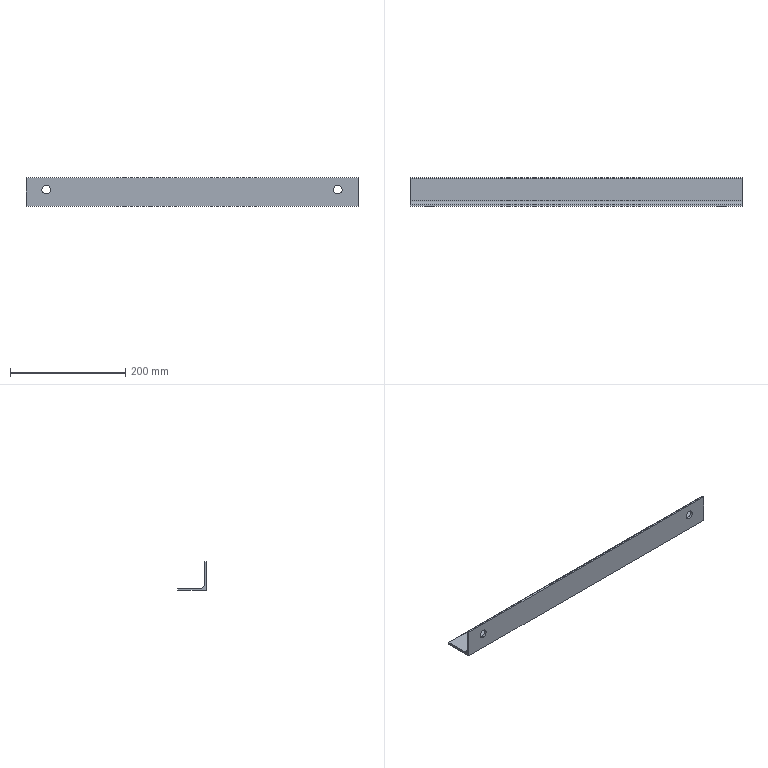Part | STEP file | 电柜通道角钢1_Default<As Machined> | 1 solid | 15 faces | box 575 x 50 x 50 mm | volume 222682 mm3 | plane 8 | cylinder 7 | commonest cylinder face diameters 15 x4 2.66 x2 11 x1
STEP:
#1=CARTESIAN_POINT('',(0.,0.,0.));
#2=DIRECTION('',(0.,0.,1.));
#3=DIRECTION('',(1.,0.,0.));
#4=AXIS2_PLACEMENT_3D('',#1,#2,#3);
#5=CARTESIAN_POINT('',(-252.5,0.,36.585));
#6=VERTEX_POINT('',#5);
#7=CARTESIAN_POINT('',(-252.5,4.,36.585));
#8=VERTEX_POINT('',#7);
#9=CARTESIAN_POINT('',(-252.5,-6.,36.585));
#10=DIRECTION('',(0.,1.,0.));
#11=VECTOR('',#10,1.);
#12=LINE('',#9,#11);
#13=CARTESIAN_POINT('',(-252.5,-6.,29.085));
#14=DIRECTION('',(0.,1.,0.));
#15=DIRECTION('',(0.,0.,1.));
#16=AXIS2_PLACEMENT_3D('',#13,#14,#15);
#17=CYLINDRICAL_SURFACE('',#16,7.5);
#18=CARTESIAN_POINT('',(6.283,0.));
#19=DIRECTION('',(0.,1.));
#20=VECTOR('',#19,1.);
#21=LINE('',#18,#20);
#22=(GEOMETRIC_REPRESENTATION_CONTEXT(2)PARAMETRIC_REPRESENTATION_CONTEXT()REPRESENTATION_CONTEXT('',''));
#23=DEFINITIONAL_REPRESENTATION('',(#21),#22);
#24=PCURVE('',#17,#23);
#25=CARTESIAN_POINT('',(-252.5,-6.,29.085));
#26=DIRECTION('',(0.,1.,0.));
#27=DIRECTION('',(0.,0.,1.));
#28=AXIS2_PLACEMENT_3D('',#25,#26,#27);
#29=CYLINDRICAL_SURFACE('',#28,7.5);
#30=CARTESIAN_POINT('',(0.,0.));
#31=DIRECTION('',(0.,1.));
#32=VECTOR('',#31,1.);
#33=LINE('',#30,#32);
#34=(GEOMETRIC_REPRESENTATION_CONTEXT(2)PARAMETRIC_REPRESENTATION_CONTEXT()REPRESENTATION_CONTEXT('',''));
#35=DEFINITIONAL_REPRESENTATION('',(#33),#34);
#36=PCURVE('',#29,#35);
#37=SURFACE_CURVE('',#12,(#24,#36),.PCURVE_S1.);
#38=EDGE_CURVE('',#6,#8,#37,.T.);
#39=ORIENTED_EDGE('',*,*,#38,.T.);
#40=CARTESIAN_POINT('',(-252.5,4.,21.585));
#41=VERTEX_POINT('',#40);
#42=CARTESIAN_POINT('',(-252.5,4.,29.085));
#43=DIRECTION('',(0.,1.,0.));
#44=DIRECTION('',(0.,0.,1.));
#45=AXIS2_PLACEMENT_3D('',#42,#43,#44);
#46=CIRCLE('',#45,7.5);
#47=CARTESIAN_POINT('',(0.,10.));
#48=DIRECTION('',(1.,0.));
#49=VECTOR('',#48,1.);
#50=LINE('',#47,#49);
#51=(GEOMETRIC_REPRESENTATION_CONTEXT(2)PARAMETRIC_REPRESENTATION_CONTEXT()REPRESENTATION_CONTEXT('',''));
#52=DEFINITIONAL_REPRESENTATION('',(#50),#51);
#53=PCURVE('',#17,#52);
#54=CARTESIAN_POINT('',(287.5,4.,48.67));
#55=DIRECTION('',(0.,-1.,0.));
#56=DIRECTION('',(1.,0.,0.));
#57=AXIS2_PLACEMENT_3D('',#54,#55,#56);
#58=PLANE('',#57);
#59=CARTESIAN_POINT('',(-540.,-12.085));
#60=CARTESIAN_POINT('',(-527.01,-12.085));
#61=CARTESIAN_POINT('',(-533.505,-23.335));
#62=CARTESIAN_POINT('',(-540.,-34.585));
#63=CARTESIAN_POINT('',(-546.495,-23.335));
#64=CARTESIAN_POINT('',(-552.99,-12.085));
#65=CARTESIAN_POINT('',(-540.,-12.085));
#66=(BOUNDED_CURVE()B_SPLINE_CURVE(2,(#59,#60,#61,#62,#63,#64,#65),.UNSPECIFIED.,.T.,.F.)B_SPLINE_CURVE_WITH_KNOTS((1,2,2,2,2,1),(-2.094,0.,2.094,4.189,6.283,8.378),.UNSPECIFIED.)CURVE()GEOMETRIC_REPRESENTATION_ITEM()RATIONAL_B_SPLINE_CURVE((1.,0.5,1.,0.5,1.,0.5,1.))REPRESENTATION_ITEM(''));
#67=(GEOMETRIC_REPRESENTATION_CONTEXT(2)PARAMETRIC_REPRESENTATION_CONTEXT()REPRESENTATION_CONTEXT('',''));
#68=DEFINITIONAL_REPRESENTATION('',(#66),#67);
#69=PCURVE('',#58,#68);
#70=SURFACE_CURVE('',#46,(#53,#69),.PCURVE_S1.);
#71=EDGE_CURVE('',#41,#8,#70,.T.);
#72=ORIENTED_EDGE('',*,*,#71,.F.);
#73=CARTESIAN_POINT('',(-252.5,0.,21.585));
#74=VERTEX_POINT('',#73);
#75=CARTESIAN_POINT('',(-252.5,-6.,21.585));
#76=DIRECTION('',(0.,1.,0.));
#77=VECTOR('',#76,1.);
#78=LINE('',#75,#77);
#79=CARTESIAN_POINT('',(3.142,0.));
#80=DIRECTION('',(0.,1.));
#81=VECTOR('',#80,1.);
#82=LINE('',#79,#81);
#83=(GEOMETRIC_REPRESENTATION_CONTEXT(2)PARAMETRIC_REPRESENTATION_CONTEXT()REPRESENTATION_CONTEXT('',''));
#84=DEFINITIONAL_REPRESENTATION('',(#82),#83);
#85=PCURVE('',#17,#84);
#86=CARTESIAN_POINT('',(3.142,0.));
#87=DIRECTION('',(0.,1.));
#88=VECTOR('',#87,1.);
#89=LINE('',#86,#88);
#90=(GEOMETRIC_REPRESENTATION_CONTEXT(2)PARAMETRIC_REPRESENTATION_CONTEXT()REPRESENTATION_CONTEXT('',''));
#91=DEFINITIONAL_REPRESENTATION('',(#89),#90);
#92=PCURVE('',#29,#91);
#93=SURFACE_CURVE('',#78,(#85,#92),.PCURVE_S1.);
#94=EDGE_CURVE('',#74,#41,#93,.T.);
#95=ORIENTED_EDGE('',*,*,#94,.F.);
#96=CARTESIAN_POINT('',(-252.5,0.,29.085));
#97=DIRECTION('',(0.,1.,0.));
#98=DIRECTION('',(-1.,0.,0.));
#99=AXIS2_PLACEMENT_3D('',#96,#97,#98);
#100=CIRCLE('',#99,7.5);
#101=CARTESIAN_POINT('',(-1.571,6.));
#102=DIRECTION('',(1.,0.));
#103=VECTOR('',#102,1.);
#104=LINE('',#101,#103);
#105=(GEOMETRIC_REPRESENTATION_CONTEXT(2)PARAMETRIC_REPRESENTATION_CONTEXT()REPRESENTATION_CONTEXT('',''));
#106=DEFINITIONAL_REPRESENTATION('',(#104),#105);
#107=PCURVE('',#17,#106);
#108=CARTESIAN_POINT('',(287.5,0.,50.));
#109=DIRECTION('',(0.,1.,0.));
#110=DIRECTION('',(-1.,0.,0.));
#111=AXIS2_PLACEMENT_3D('',#108,#109,#110);
#112=PLANE('',#111);
#113=CARTESIAN_POINT('',(540.,-20.915));
#114=DIRECTION('',(1.,0.));
#115=AXIS2_PLACEMENT_2D('',#113,#114);
#116=CIRCLE('',#115,7.5);
#117=(GEOMETRIC_REPRESENTATION_CONTEXT(2)PARAMETRIC_REPRESENTATION_CONTEXT()REPRESENTATION_CONTEXT('',''));
#118=DEFINITIONAL_REPRESENTATION('',(#116),#117);
#119=PCURVE('',#112,#118);
#120=SURFACE_CURVE('',#100,(#107,#119),.PCURVE_S1.);
#121=EDGE_CURVE('',#74,#6,#120,.T.);
#122=ORIENTED_EDGE('',*,*,#121,.T.);
#123=EDGE_LOOP('',(#39,#72,#95,#122));
#124=FACE_BOUND('',#123,.F.);
#125=ADVANCED_FACE('',(#124),#17,.F.);
#126=CARTESIAN_POINT('',(252.5,0.,36.585));
#127=VERTEX_POINT('',#126);
#128=CARTESIAN_POINT('',(252.5,4.,36.585));
#129=VERTEX_POINT('',#128);
#130=CARTESIAN_POINT('',(252.5,-6.,36.585));
#131=DIRECTION('',(0.,1.,0.));
#132=VECTOR('',#131,1.);
#133=LINE('',#130,#132);
#134=CARTESIAN_POINT('',(252.5,-6.,29.085));
#135=DIRECTION('',(0.,1.,0.));
#136=DIRECTION('',(0.,0.,1.));
#137=AXIS2_PLACEMENT_3D('',#134,#135,#136);
#138=CYLINDRICAL_SURFACE('',#137,7.5);
#139=CARTESIAN_POINT('',(6.283,0.));
#140=DIRECTION('',(0.,1.));
#141=VECTOR('',#140,1.);
#142=LINE('',#139,#141);
#143=(GEOMETRIC_REPRESENTATION_CONTEXT(2)PARAMETRIC_REPRESENTATION_CONTEXT()REPRESENTATION_CONTEXT('',''));
#144=DEFINITIONAL_REPRESENTATION('',(#142),#143);
#145=PCURVE('',#138,#144);
#146=CARTESIAN_POINT('',(252.5,-6.,29.085));
#147=DIRECTION('',(0.,1.,0.));
#148=DIRECTION('',(0.,0.,1.));
#149=AXIS2_PLACEMENT_3D('',#146,#147,#148);
#150=CYLINDRICAL_SURFACE('',#149,7.5);
#151=CARTESIAN_POINT('',(0.,0.));
#152=DIRECTION('',(0.,1.));
#153=VECTOR('',#152,1.);
#154=LINE('',#151,#153);
#155=(GEOMETRIC_REPRESENTATION_CONTEXT(2)PARAMETRIC_REPRESENTATION_CONTEXT()REPRESENTATION_CONTEXT('',''));
#156=DEFINITIONAL_REPRESENTATION('',(#154),#155);
#157=PCURVE('',#150,#156);
#158=SURFACE_CURVE('',#133,(#145,#157),.PCURVE_S1.);
#159=EDGE_CURVE('',#127,#129,#158,.T.);
#160=ORIENTED_EDGE('',*,*,#159,.T.);
#161=CARTESIAN_POINT('',(252.5,4.,21.585));
#162=VERTEX_POINT('',#161);
#163=CARTESIAN_POINT('',(252.5,4.,29.085));
#164=DIRECTION('',(0.,1.,0.));
#165=DIRECTION('',(0.,0.,-1.));
#166=AXIS2_PLACEMENT_3D('',#163,#164,#165);
#167=CIRCLE('',#166,7.5);
#168=CARTESIAN_POINT('',(3.142,10.));
#169=DIRECTION('',(1.,0.));
#170=VECTOR('',#169,1.);
#171=LINE('',#168,#170);
#172=(GEOMETRIC_REPRESENTATION_CONTEXT(2)PARAMETRIC_REPRESENTATION_CONTEXT()REPRESENTATION_CONTEXT('',''));
#173=DEFINITIONAL_REPRESENTATION('',(#171),#172);
#174=PCURVE('',#138,#173);
#175=CARTESIAN_POINT('',(-35.,-27.085));
#176=CARTESIAN_POINT('',(-47.99,-27.085));
#177=CARTESIAN_POINT('',(-41.495,-15.835));
#178=CARTESIAN_POINT('',(-35.,-4.585));
#179=CARTESIAN_POINT('',(-28.505,-15.835));
#180=CARTESIAN_POINT('',(-22.01,-27.085));
#181=CARTESIAN_POINT('',(-35.,-27.085));
#182=(BOUNDED_CURVE()B_SPLINE_CURVE(2,(#175,#176,#177,#178,#179,#180,#181),.UNSPECIFIED.,.T.,.F.)B_SPLINE_CURVE_WITH_KNOTS((1,2,2,2,2,1),(-2.094,0.,2.094,4.189,6.283,8.378),.UNSPECIFIED.)CURVE()GEOMETRIC_REPRESENTATION_ITEM()RATIONAL_B_SPLINE_CURVE((1.,0.5,1.,0.5,1.,0.5,1.))REPRESENTATION_ITEM(''));
#183=(GEOMETRIC_REPRESENTATION_CONTEXT(2)PARAMETRIC_REPRESENTATION_CONTEXT()REPRESENTATION_CONTEXT('',''));
#184=DEFINITIONAL_REPRESENTATION('',(#182),#183);
#185=PCURVE('',#58,#184);
#186=SURFACE_CURVE('',#167,(#174,#185),.PCURVE_S1.);
#187=EDGE_CURVE('',#162,#129,#186,.T.);
#188=ORIENTED_EDGE('',*,*,#187,.F.);
#189=CARTESIAN_POINT('',(252.5,0.,21.585));
#190=VERTEX_POINT('',#189);
#191=CARTESIAN_POINT('',(252.5,-6.,21.585));
#192=DIRECTION('',(0.,1.,0.));
#193=VECTOR('',#192,1.);
#194=LINE('',#191,#193);
#195=CARTESIAN_POINT('',(3.142,0.));
#196=DIRECTION('',(0.,1.));
#197=VECTOR('',#196,1.);
#198=LINE('',#195,#197);
#199=(GEOMETRIC_REPRESENTATION_CONTEXT(2)PARAMETRIC_REPRESENTATION_CONTEXT()REPRESENTATION_CONTEXT('',''));
#200=DEFINITIONAL_REPRESENTATION('',(#198),#199);
#201=PCURVE('',#138,#200);
#202=CARTESIAN_POINT('',(3.142,0.));
#203=DIRECTION('',(0.,1.));
#204=VECTOR('',#203,1.);
#205=LINE('',#202,#204);
#206=(GEOMETRIC_REPRESENTATION_CONTEXT(2)PARAMETRIC_REPRESENTATION_CONTEXT()REPRESENTATION_CONTEXT('',''));
#207=DEFINITIONAL_REPRESENTATION('',(#205),#206);
#208=PCURVE('',#150,#207);
#209=SURFACE_CURVE('',#194,(#201,#208),.PCURVE_S1.);
#210=EDGE_CURVE('',#190,#162,#209,.T.);
#211=ORIENTED_EDGE('',*,*,#210,.F.);
#212=CARTESIAN_POINT('',(252.5,0.,29.085));
#213=DIRECTION('',(0.,1.,0.));
#214=DIRECTION('',(-1.,0.,0.));
#215=AXIS2_PLACEMENT_3D('',#212,#213,#214);
#216=CIRCLE('',#215,7.5);
#217=CARTESIAN_POINT('',(-1.571,6.));
#218=DIRECTION('',(1.,0.));
#219=VECTOR('',#218,1.);
#220=LINE('',#217,#219);
#221=(GEOMETRIC_REPRESENTATION_CONTEXT(2)PARAMETRIC_REPRESENTATION_CONTEXT()REPRESENTATION_CONTEXT('',''));
#222=DEFINITIONAL_REPRESENTATION('',(#220),#221);
#223=PCURVE('',#138,#222);
#224=CARTESIAN_POINT('',(35.,-20.915));
#225=DIRECTION('',(1.,0.));
#226=AXIS2_PLACEMENT_2D('',#224,#225);
#227=CIRCLE('',#226,7.5);
#228=(GEOMETRIC_REPRESENTATION_CONTEXT(2)PARAMETRIC_REPRESENTATION_CONTEXT()REPRESENTATION_CONTEXT('',''));
#229=DEFINITIONAL_REPRESENTATION('',(#227),#228);
#230=PCURVE('',#112,#229);
#231=SURFACE_CURVE('',#216,(#223,#230),.PCURVE_S1.);
#232=EDGE_CURVE('',#190,#127,#231,.T.);
#233=ORIENTED_EDGE('',*,*,#232,.T.);
#234=EDGE_LOOP('',(#160,#188,#211,#233));
#235=FACE_BOUND('',#234,.F.);
#236=ADVANCED_FACE('',(#235),#138,.F.);
#237=CARTESIAN_POINT('',(-287.5,50.,2.67));
#238=VERTEX_POINT('',#237);
#239=CARTESIAN_POINT('',(-287.5,48.67,4.));
#240=VERTEX_POINT('',#239);
#241=CARTESIAN_POINT('',(-287.5,48.67,2.67));
#242=DIRECTION('',(1.,0.,0.));
#243=DIRECTION('',(0.,1.,0.));
#244=AXIS2_PLACEMENT_3D('',#241,#242,#243);
#245=CIRCLE('',#244,1.33);
#246=CARTESIAN_POINT('',(287.5,48.67,2.67));
#247=DIRECTION('',(-1.,0.,0.));
#248=DIRECTION('',(0.,-1.,0.));
#249=AXIS2_PLACEMENT_3D('',#246,#247,#248);
#250=CYLINDRICAL_SURFACE('',#249,1.33);
#251=CARTESIAN_POINT('',(3.142,575.));
#252=DIRECTION('',(-1.,0.));
#253=VECTOR('',#252,1.);
#254=LINE('',#251,#253);
#255=(GEOMETRIC_REPRESENTATION_CONTEXT(2)PARAMETRIC_REPRESENTATION_CONTEXT()REPRESENTATION_CONTEXT('',''));
#256=DEFINITIONAL_REPRESENTATION('',(#254),#255);
#257=PCURVE('',#250,#256);
#258=CARTESIAN_POINT('',(-287.5,48.67,2.67));
#259=DIRECTION('',(1.,0.,0.));
#260=DIRECTION('',(0.,1.,0.));
#261=AXIS2_PLACEMENT_3D('',#258,#259,#260);
#262=PLANE('',#261);
#263=CARTESIAN_POINT('',(0.,0.));
#264=DIRECTION('',(1.,0.));
#265=AXIS2_PLACEMENT_2D('',#263,#264);
#266=CIRCLE('',#265,1.33);
#267=(GEOMETRIC_REPRESENTATION_CONTEXT(2)PARAMETRIC_REPRESENTATION_CONTEXT()REPRESENTATION_CONTEXT('',''));
#268=DEFINITIONAL_REPRESENTATION('',(#266),#267);
#269=PCURVE('',#262,#268);
#270=SURFACE_CURVE('',#245,(#257,#269),.PCURVE_S1.);
#271=EDGE_CURVE('',#238,#240,#270,.T.);
#272=ORIENTED_EDGE('',*,*,#271,.T.);
#273=CARTESIAN_POINT('',(287.5,48.67,4.));
#274=VERTEX_POINT('',#273);
#275=CARTESIAN_POINT('',(287.5,48.67,4.));
#276=DIRECTION('',(-1.,0.,0.));
#277=VECTOR('',#276,1.);
#278=LINE('',#275,#277);
#279=CARTESIAN_POINT('',(1.571,0.));
#280=DIRECTION('',(0.,1.));
#281=VECTOR('',#280,1.);
#282=LINE('',#279,#281);
#283=(GEOMETRIC_REPRESENTATION_CONTEXT(2)PARAMETRIC_REPRESENTATION_CONTEXT()REPRESENTATION_CONTEXT('',''));
#284=DEFINITIONAL_REPRESENTATION('',(#282),#283);
#285=PCURVE('',#250,#284);
#286=CARTESIAN_POINT('',(287.5,9.5,4.));
#287=DIRECTION('',(0.,0.,-1.));
#288=DIRECTION('',(-1.,0.,0.));
#289=AXIS2_PLACEMENT_3D('',#286,#287,#288);
#290=PLANE('',#289);
#291=CARTESIAN_POINT('',(0.,39.17));
#292=DIRECTION('',(1.,0.));
#293=VECTOR('',#292,1.);
#294=LINE('',#291,#293);
#295=(GEOMETRIC_REPRESENTATION_CONTEXT(2)PARAMETRIC_REPRESENTATION_CONTEXT()REPRESENTATION_CONTEXT('',''));
#296=DEFINITIONAL_REPRESENTATION('',(#294),#295);
#297=PCURVE('',#290,#296);
#298=SURFACE_CURVE('',#278,(#285,#297),.PCURVE_S1.);
#299=EDGE_CURVE('',#274,#240,#298,.T.);
#300=ORIENTED_EDGE('',*,*,#299,.F.);
#301=CARTESIAN_POINT('',(287.5,50.,2.67));
#302=VERTEX_POINT('',#301);
#303=CARTESIAN_POINT('',(287.5,48.67,2.67));
#304=DIRECTION('',(1.,0.,0.));
#305=DIRECTION('',(0.,1.,0.));
#306=AXIS2_PLACEMENT_3D('',#303,#304,#305);
#307=CIRCLE('',#306,1.33);
#308=CARTESIAN_POINT('',(3.142,0.));
#309=DIRECTION('',(-1.,0.));
#310=VECTOR('',#309,1.);
#311=LINE('',#308,#310);
#312=(GEOMETRIC_REPRESENTATION_CONTEXT(2)PARAMETRIC_REPRESENTATION_CONTEXT()REPRESENTATION_CONTEXT('',''));
#313=DEFINITIONAL_REPRESENTATION('',(#311),#312);
#314=PCURVE('',#250,#313);
#315=CARTESIAN_POINT('',(287.5,48.67,2.67));
#316=DIRECTION('',(1.,0.,0.));
#317=DIRECTION('',(0.,1.,0.));
#318=AXIS2_PLACEMENT_3D('',#315,#316,#317);
#319=PLANE('',#318);
#320=CARTESIAN_POINT('',(0.,0.));
#321=DIRECTION('',(1.,0.));
#322=AXIS2_PLACEMENT_2D('',#320,#321);
#323=CIRCLE('',#322,1.33);
#324=(GEOMETRIC_REPRESENTATION_CONTEXT(2)PARAMETRIC_REPRESENTATION_CONTEXT()REPRESENTATION_CONTEXT('',''));
#325=DEFINITIONAL_REPRESENTATION('',(#323),#324);
#326=PCURVE('',#319,#325);
#327=SURFACE_CURVE('',#307,(#314,#326),.PCURVE_S1.);
#328=EDGE_CURVE('',#302,#274,#327,.T.);
#329=ORIENTED_EDGE('',*,*,#328,.F.);
#330=CARTESIAN_POINT('',(287.5,50.,2.67));
#331=DIRECTION('',(-1.,0.,0.));
#332=VECTOR('',#331,1.);
#333=LINE('',#330,#332);
#334=CARTESIAN_POINT('',(3.142,0.));
#335=DIRECTION('',(0.,1.));
#336=VECTOR('',#335,1.);
#337=LINE('',#334,#336);
#338=(GEOMETRIC_REPRESENTATION_CONTEXT(2)PARAMETRIC_REPRESENTATION_CONTEXT()REPRESENTATION_CONTEXT('',''));
#339=DEFINITIONAL_REPRESENTATION('',(#337),#338);
#340=PCURVE('',#250,#339);
#341=CARTESIAN_POINT('',(287.5,50.,2.67));
#342=DIRECTION('',(0.,-1.,0.));
#343=DIRECTION('',(1.,0.,0.));
#344=AXIS2_PLACEMENT_3D('',#341,#342,#343);
#345=PLANE('',#344);
#346=CARTESIAN_POINT('',(0.,0.));
#347=DIRECTION('',(-1.,0.));
#348=VECTOR('',#347,1.);
#349=LINE('',#346,#348);
#350=(GEOMETRIC_REPRESENTATION_CONTEXT(2)PARAMETRIC_REPRESENTATION_CONTEXT()REPRESENTATION_CONTEXT('',''));
#351=DEFINITIONAL_REPRESENTATION('',(#349),#350);
#352=PCURVE('',#345,#351);
#353=SURFACE_CURVE('',#333,(#340,#352),.PCURVE_S1.);
#354=EDGE_CURVE('',#302,#238,#353,.T.);
#355=ORIENTED_EDGE('',*,*,#354,.T.);
#356=EDGE_LOOP('',(#272,#300,#329,#355));
#357=FACE_BOUND('',#356,.T.);
#358=ADVANCED_FACE('',(#357),#250,.T.);
#359=CARTESIAN_POINT('',(-287.5,9.5,4.));
#360=VERTEX_POINT('',#359);
#361=CARTESIAN_POINT('',(-287.5,9.5,4.));
#362=DIRECTION('',(0.,-1.,0.));
#363=VECTOR('',#362,1.);
#364=LINE('',#361,#363);
#365=CARTESIAN_POINT('',(575.,0.));
#366=DIRECTION('',(0.,-1.));
#367=VECTOR('',#366,1.);
#368=LINE('',#365,#367);
#369=(GEOMETRIC_REPRESENTATION_CONTEXT(2)PARAMETRIC_REPRESENTATION_CONTEXT()REPRESENTATION_CONTEXT('',''));
#370=DEFINITIONAL_REPRESENTATION('',(#368),#369);
#371=PCURVE('',#290,#370);
#372=CARTESIAN_POINT('',(-39.17,1.33));
#373=DIRECTION('',(-1.,0.));
#374=VECTOR('',#373,1.);
#375=LINE('',#372,#374);
#376=(GEOMETRIC_REPRESENTATION_CONTEXT(2)PARAMETRIC_REPRESENTATION_CONTEXT()REPRESENTATION_CONTEXT('',''));
#377=DEFINITIONAL_REPRESENTATION('',(#375),#376);
#378=PCURVE('',#262,#377);
#379=SURFACE_CURVE('',#364,(#371,#378),.PCURVE_S1.);
#380=EDGE_CURVE('',#240,#360,#379,.T.);
#381=ORIENTED_EDGE('',*,*,#380,.T.);
#382=CARTESIAN_POINT('',(287.5,9.5,4.));
#383=VERTEX_POINT('',#382);
#384=CARTESIAN_POINT('',(287.5,9.5,4.));
#385=DIRECTION('',(-1.,0.,0.));
#386=VECTOR('',#385,1.);
#387=LINE('',#384,#386);
#388=CARTESIAN_POINT('',(0.,0.));
#389=DIRECTION('',(1.,0.));
#390=VECTOR('',#389,1.);
#391=LINE('',#388,#390);
#392=(GEOMETRIC_REPRESENTATION_CONTEXT(2)PARAMETRIC_REPRESENTATION_CONTEXT()REPRESENTATION_CONTEXT('',''));
#393=DEFINITIONAL_REPRESENTATION('',(#391),#392);
#394=PCURVE('',#290,#393);
#395=CARTESIAN_POINT('',(287.5,9.5,9.5));
#396=DIRECTION('',(-1.,0.,0.));
#397=DIRECTION('',(0.,-1.,0.));
#398=AXIS2_PLACEMENT_3D('',#395,#396,#397);
#399=CYLINDRICAL_SURFACE('',#398,5.5);
#400=CARTESIAN_POINT('',(4.712,0.));
#401=DIRECTION('',(0.,1.));
#402=VECTOR('',#401,1.);
#403=LINE('',#400,#402);
#404=(GEOMETRIC_REPRESENTATION_CONTEXT(2)PARAMETRIC_REPRESENTATION_CONTEXT()REPRESENTATION_CONTEXT('',''));
#405=DEFINITIONAL_REPRESENTATION('',(#403),#404);
#406=PCURVE('',#399,#405);
#407=SURFACE_CURVE('',#387,(#394,#406),.PCURVE_S1.);
#408=EDGE_CURVE('',#383,#360,#407,.T.);
#409=ORIENTED_EDGE('',*,*,#408,.F.);
#410=CARTESIAN_POINT('',(287.5,9.5,4.));
#411=DIRECTION('',(0.,-1.,0.));
#412=VECTOR('',#411,1.);
#413=LINE('',#410,#412);
#414=CARTESIAN_POINT('',(0.,0.));
#415=DIRECTION('',(0.,-1.));
#416=VECTOR('',#415,1.);
#417=LINE('',#414,#416);
#418=(GEOMETRIC_REPRESENTATION_CONTEXT(2)PARAMETRIC_REPRESENTATION_CONTEXT()REPRESENTATION_CONTEXT('',''));
#419=DEFINITIONAL_REPRESENTATION('',(#417),#418);
#420=PCURVE('',#290,#419);
#421=CARTESIAN_POINT('',(-39.17,1.33));
#422=DIRECTION('',(-1.,0.));
#423=VECTOR('',#422,1.);
#424=LINE('',#421,#423);
#425=(GEOMETRIC_REPRESENTATION_CONTEXT(2)PARAMETRIC_REPRESENTATION_CONTEXT()REPRESENTATION_CONTEXT('',''));
#426=DEFINITIONAL_REPRESENTATION('',(#424),#425);
#427=PCURVE('',#319,#426);
#428=SURFACE_CURVE('',#413,(#420,#427),.PCURVE_S1.);
#429=EDGE_CURVE('',#274,#383,#428,.T.);
#430=ORIENTED_EDGE('',*,*,#429,.F.);
#431=ORIENTED_EDGE('',*,*,#299,.T.);
#432=EDGE_LOOP('',(#381,#409,#430,#431));
#433=FACE_BOUND('',#432,.T.);
#434=ADVANCED_FACE('',(#433),#290,.F.);
#435=ORIENTED_EDGE('',*,*,#408,.F.);
#436=CARTESIAN_POINT('',(287.5,4.,9.5));
#437=VERTEX_POINT('',#436);
#438=CARTESIAN_POINT('',(287.5,9.5,9.5));
#439=DIRECTION('',(-1.,0.,0.));
#440=DIRECTION('',(0.,1.,0.));
#441=AXIS2_PLACEMENT_3D('',#438,#439,#440);
#442=CIRCLE('',#441,5.5);
#443=CARTESIAN_POINT('',(3.142,0.));
#444=DIRECTION('',(1.,0.));
#445=VECTOR('',#444,1.);
#446=LINE('',#443,#445);
#447=(GEOMETRIC_REPRESENTATION_CONTEXT(2)PARAMETRIC_REPRESENTATION_CONTEXT()REPRESENTATION_CONTEXT('',''));
#448=DEFINITIONAL_REPRESENTATION('',(#446),#447);
#449=PCURVE('',#399,#448);
#450=CARTESIAN_POINT('',(-33.67,6.83));
#451=CARTESIAN_POINT('',(-33.67,-2.696));
#452=CARTESIAN_POINT('',(-41.92,2.067));
#453=CARTESIAN_POINT('',(-50.17,6.83));
#454=CARTESIAN_POINT('',(-41.92,11.593));
#455=CARTESIAN_POINT('',(-33.67,16.356));
#456=CARTESIAN_POINT('',(-33.67,6.83));
#457=(BOUNDED_CURVE()B_SPLINE_CURVE(2,(#450,#451,#452,#453,#454,#455,#456),.UNSPECIFIED.,.T.,.F.)B_SPLINE_CURVE_WITH_KNOTS((1,2,2,2,2,1),(-2.094,0.,2.094,4.189,6.283,8.378),.UNSPECIFIED.)CURVE()GEOMETRIC_REPRESENTATION_ITEM()RATIONAL_B_SPLINE_CURVE((1.,0.5,1.,0.5,1.,0.5,1.))REPRESENTATION_ITEM(''));
#458=(GEOMETRIC_REPRESENTATION_CONTEXT(2)PARAMETRIC_REPRESENTATION_CONTEXT()REPRESENTATION_CONTEXT('',''));
#459=DEFINITIONAL_REPRESENTATION('',(#457),#458);
#460=PCURVE('',#319,#459);
#461=SURFACE_CURVE('',#442,(#449,#460),.PCURVE_S1.);
#462=EDGE_CURVE('',#383,#437,#461,.T.);
#463=ORIENTED_EDGE('',*,*,#462,.T.);
#464=CARTESIAN_POINT('',(-287.5,4.,9.5));
#465=VERTEX_POINT('',#464);
#466=CARTESIAN_POINT('',(287.5,4.,9.5));
#467=DIRECTION('',(-1.,0.,0.));
#468=VECTOR('',#467,1.);
#469=LINE('',#466,#468);
#470=CARTESIAN_POINT('',(6.283,0.));
#471=DIRECTION('',(0.,1.));
#472=VECTOR('',#471,1.);
#473=LINE('',#470,#472);
#474=(GEOMETRIC_REPRESENTATION_CONTEXT(2)PARAMETRIC_REPRESENTATION_CONTEXT()REPRESENTATION_CONTEXT('',''));
#475=DEFINITIONAL_REPRESENTATION('',(#473),#474);
#476=PCURVE('',#399,#475);
#477=CARTESIAN_POINT('',(0.,-39.17));
#478=DIRECTION('',(-1.,0.));
#479=VECTOR('',#478,1.);
#480=LINE('',#477,#479);
#481=(GEOMETRIC_REPRESENTATION_CONTEXT(2)PARAMETRIC_REPRESENTATION_CONTEXT()REPRESENTATION_CONTEXT('',''));
#482=DEFINITIONAL_REPRESENTATION('',(#480),#481);
#483=PCURVE('',#58,#482);
#484=SURFACE_CURVE('',#469,(#476,#483),.PCURVE_S1.);
#485=EDGE_CURVE('',#437,#465,#484,.T.);
#486=ORIENTED_EDGE('',*,*,#485,.T.);
#487=CARTESIAN_POINT('',(-287.5,9.5,9.5));
#488=DIRECTION('',(-1.,0.,0.));
#489=DIRECTION('',(0.,1.,0.));
#490=AXIS2_PLACEMENT_3D('',#487,#488,#489);
#491=CIRCLE('',#490,5.5);
#492=CARTESIAN_POINT('',(3.142,575.));
#493=DIRECTION('',(1.,0.));
#494=VECTOR('',#493,1.);
#495=LINE('',#492,#494);
#496=(GEOMETRIC_REPRESENTATION_CONTEXT(2)PARAMETRIC_REPRESENTATION_CONTEXT()REPRESENTATION_CONTEXT('',''));
#497=DEFINITIONAL_REPRESENTATION('',(#495),#496);
#498=PCURVE('',#399,#497);
#499=CARTESIAN_POINT('',(-33.67,6.83));
#500=CARTESIAN_POINT('',(-33.67,-2.696));
#501=CARTESIAN_POINT('',(-41.92,2.067));
#502=CARTESIAN_POINT('',(-50.17,6.83));
#503=CARTESIAN_POINT('',(-41.92,11.593));
#504=CARTESIAN_POINT('',(-33.67,16.356));
#505=CARTESIAN_POINT('',(-33.67,6.83));
#506=(BOUNDED_CURVE()B_SPLINE_CURVE(2,(#499,#500,#501,#502,#503,#504,#505),.UNSPECIFIED.,.T.,.F.)B_SPLINE_CURVE_WITH_KNOTS((1,2,2,2,2,1),(-2.094,0.,2.094,4.189,6.283,8.378),.UNSPECIFIED.)CURVE()GEOMETRIC_REPRESENTATION_ITEM()RATIONAL_B_SPLINE_CURVE((1.,0.5,1.,0.5,1.,0.5,1.))REPRESENTATION_ITEM(''));
#507=(GEOMETRIC_REPRESENTATION_CONTEXT(2)PARAMETRIC_REPRESENTATION_CONTEXT()REPRESENTATION_CONTEXT('',''));
#508=DEFINITIONAL_REPRESENTATION('',(#506),#507);
#509=PCURVE('',#262,#508);
#510=SURFACE_CURVE('',#491,(#498,#509),.PCURVE_S1.);
#511=EDGE_CURVE('',#360,#465,#510,.T.);
#512=ORIENTED_EDGE('',*,*,#511,.F.);
#513=EDGE_LOOP('',(#435,#463,#486,#512));
#514=FACE_BOUND('',#513,.F.);
#515=ADVANCED_FACE('',(#514),#399,.F.);
#516=CARTESIAN_POINT('',(-252.5,4.,29.085));
#517=DIRECTION('',(0.,1.,0.));
#518=DIRECTION('',(0.,0.,1.));
#519=AXIS2_PLACEMENT_3D('',#516,#517,#518);
#520=CIRCLE('',#519,7.5);
#521=CARTESIAN_POINT('',(-540.,-12.085));
#522=CARTESIAN_POINT('',(-527.01,-12.085));
#523=CARTESIAN_POINT('',(-533.505,-23.335));
#524=CARTESIAN_POINT('',(-540.,-34.585));
#525=CARTESIAN_POINT('',(-546.495,-23.335));
#526=CARTESIAN_POINT('',(-552.99,-12.085));
#527=CARTESIAN_POINT('',(-540.,-12.085));
#528=(BOUNDED_CURVE()B_SPLINE_CURVE(2,(#521,#522,#523,#524,#525,#526,#527),.UNSPECIFIED.,.T.,.F.)B_SPLINE_CURVE_WITH_KNOTS((1,2,2,2,2,1),(-2.094,0.,2.094,4.189,6.283,8.378),.UNSPECIFIED.)CURVE()GEOMETRIC_REPRESENTATION_ITEM()RATIONAL_B_SPLINE_CURVE((1.,0.5,1.,0.5,1.,0.5,1.))REPRESENTATION_ITEM(''));
#529=(GEOMETRIC_REPRESENTATION_CONTEXT(2)PARAMETRIC_REPRESENTATION_CONTEXT()REPRESENTATION_CONTEXT('',''));
#530=DEFINITIONAL_REPRESENTATION('',(#528),#529);
#531=PCURVE('',#58,#530);
#532=CARTESIAN_POINT('',(0.,10.));
#533=DIRECTION('',(1.,0.));
#534=VECTOR('',#533,1.);
#535=LINE('',#532,#534);
#536=(GEOMETRIC_REPRESENTATION_CONTEXT(2)PARAMETRIC_REPRESENTATION_CONTEXT()REPRESENTATION_CONTEXT('',''));
#537=DEFINITIONAL_REPRESENTATION('',(#535),#536);
#538=PCURVE('',#29,#537);
#539=SURFACE_CURVE('',#520,(#531,#538),.PCURVE_S1.);
#540=EDGE_CURVE('',#8,#41,#539,.T.);
#541=ORIENTED_EDGE('',*,*,#540,.F.);
#542=ORIENTED_EDGE('',*,*,#71,.F.);
#543=EDGE_LOOP('',(#541,#542));
#544=FACE_BOUND('',#543,.T.);
#545=CARTESIAN_POINT('',(252.5,4.,29.085));
#546=DIRECTION('',(0.,1.,0.));
#547=DIRECTION('',(0.,0.,-1.));
#548=AXIS2_PLACEMENT_3D('',#545,#546,#547);
#549=CIRCLE('',#548,7.5);
#550=CARTESIAN_POINT('',(-35.,-27.085));
#551=CARTESIAN_POINT('',(-47.99,-27.085));
#552=CARTESIAN_POINT('',(-41.495,-15.835));
#553=CARTESIAN_POINT('',(-35.,-4.585));
#554=CARTESIAN_POINT('',(-28.505,-15.835));
#555=CARTESIAN_POINT('',(-22.01,-27.085));
#556=CARTESIAN_POINT('',(-35.,-27.085));
#557=(BOUNDED_CURVE()B_SPLINE_CURVE(2,(#550,#551,#552,#553,#554,#555,#556),.UNSPECIFIED.,.T.,.F.)B_SPLINE_CURVE_WITH_KNOTS((1,2,2,2,2,1),(-2.094,0.,2.094,4.189,6.283,8.378),.UNSPECIFIED.)CURVE()GEOMETRIC_REPRESENTATION_ITEM()RATIONAL_B_SPLINE_CURVE((1.,0.5,1.,0.5,1.,0.5,1.))REPRESENTATION_ITEM(''));
#558=(GEOMETRIC_REPRESENTATION_CONTEXT(2)PARAMETRIC_REPRESENTATION_CONTEXT()REPRESENTATION_CONTEXT('',''));
#559=DEFINITIONAL_REPRESENTATION('',(#557),#558);
#560=PCURVE('',#58,#559);
#561=CARTESIAN_POINT('',(-3.142,10.));
#562=DIRECTION('',(1.,0.));
#563=VECTOR('',#562,1.);
#564=LINE('',#561,#563);
#565=(GEOMETRIC_REPRESENTATION_CONTEXT(2)PARAMETRIC_REPRESENTATION_CONTEXT()REPRESENTATION_CONTEXT('',''));
#566=DEFINITIONAL_REPRESENTATION('',(#564),#565);
#567=PCURVE('',#150,#566);
#568=SURFACE_CURVE('',#549,(#560,#567),.PCURVE_S1.);
#569=EDGE_CURVE('',#129,#162,#568,.T.);
#570=ORIENTED_EDGE('',*,*,#569,.F.);
#571=ORIENTED_EDGE('',*,*,#187,.F.);
#572=EDGE_LOOP('',(#570,#571));
#573=FACE_BOUND('',#572,.T.);
#574=CARTESIAN_POINT('',(-287.5,4.,48.67));
#575=VERTEX_POINT('',#574);
#576=CARTESIAN_POINT('',(-287.5,4.,48.67));
#577=DIRECTION('',(0.,0.,1.));
#578=VECTOR('',#577,1.);
#579=LINE('',#576,#578);
#580=CARTESIAN_POINT('',(-575.,0.));
#581=DIRECTION('',(0.,1.));
#582=VECTOR('',#581,1.);
#583=LINE('',#580,#582);
#584=(GEOMETRIC_REPRESENTATION_CONTEXT(2)PARAMETRIC_REPRESENTATION_CONTEXT()REPRESENTATION_CONTEXT('',''));
#585=DEFINITIONAL_REPRESENTATION('',(#583),#584);
#586=PCURVE('',#58,#585);
#587=CARTESIAN_POINT('',(-44.67,46.));
#588=DIRECTION('',(0.,1.));
#589=VECTOR('',#588,1.);
#590=LINE('',#587,#589);
#591=(GEOMETRIC_REPRESENTATION_CONTEXT(2)PARAMETRIC_REPRESENTATION_CONTEXT()REPRESENTATION_CONTEXT('',''));
#592=DEFINITIONAL_REPRESENTATION('',(#590),#591);
#593=PCURVE('',#262,#592);
#594=SURFACE_CURVE('',#579,(#586,#593),.PCURVE_S1.);
#595=EDGE_CURVE('',#465,#575,#594,.T.);
#596=ORIENTED_EDGE('',*,*,#595,.T.);
#597=CARTESIAN_POINT('',(287.5,4.,48.67));
#598=VERTEX_POINT('',#597);
#599=CARTESIAN_POINT('',(287.5,4.,48.67));
#600=DIRECTION('',(-1.,0.,0.));
#601=VECTOR('',#600,1.);
#602=LINE('',#599,#601);
#603=CARTESIAN_POINT('',(0.,0.));
#604=DIRECTION('',(-1.,0.));
#605=VECTOR('',#604,1.);
#606=LINE('',#603,#605);
#607=(GEOMETRIC_REPRESENTATION_CONTEXT(2)PARAMETRIC_REPRESENTATION_CONTEXT()REPRESENTATION_CONTEXT('',''));
#608=DEFINITIONAL_REPRESENTATION('',(#606),#607);
#609=PCURVE('',#58,#608);
#610=CARTESIAN_POINT('',(287.5,2.67,48.67));
#611=DIRECTION('',(-1.,0.,0.));
#612=DIRECTION('',(0.,-1.,0.));
#613=AXIS2_PLACEMENT_3D('',#610,#611,#612);
#614=CYLINDRICAL_SURFACE('',#613,1.33);
#615=CARTESIAN_POINT('',(3.142,0.));
#616=DIRECTION('',(0.,1.));
#617=VECTOR('',#616,1.);
#618=LINE('',#615,#617);
#619=(GEOMETRIC_REPRESENTATION_CONTEXT(2)PARAMETRIC_REPRESENTATION_CONTEXT()REPRESENTATION_CONTEXT('',''));
#620=DEFINITIONAL_REPRESENTATION('',(#618),#619);
#621=PCURVE('',#614,#620);
#622=SURFACE_CURVE('',#602,(#609,#621),.PCURVE_S1.);
#623=EDGE_CURVE('',#598,#575,#622,.T.);
#624=ORIENTED_EDGE('',*,*,#623,.F.);
#625=CARTESIAN_POINT('',(287.5,4.,48.67));
#626=DIRECTION('',(0.,0.,1.));
#627=VECTOR('',#626,1.);
#628=LINE('',#625,#627);
#629=CARTESIAN_POINT('',(0.,0.));
#630=DIRECTION('',(0.,1.));
#631=VECTOR('',#630,1.);
#632=LINE('',#629,#631);
#633=(GEOMETRIC_REPRESENTATION_CONTEXT(2)PARAMETRIC_REPRESENTATION_CONTEXT()REPRESENTATION_CONTEXT('',''));
#634=DEFINITIONAL_REPRESENTATION('',(#632),#633);
#635=PCURVE('',#58,#634);
#636=CARTESIAN_POINT('',(-44.67,46.));
#637=DIRECTION('',(0.,1.));
#638=VECTOR('',#637,1.);
#639=LINE('',#636,#638);
#640=(GEOMETRIC_REPRESENTATION_CONTEXT(2)PARAMETRIC_REPRESENTATION_CONTEXT()REPRESENTATION_CONTEXT('',''));
#641=DEFINITIONAL_REPRESENTATION('',(#639),#640);
#642=PCURVE('',#319,#641);
#643=SURFACE_CURVE('',#628,(#635,#642),.PCURVE_S1.);
#644=EDGE_CURVE('',#437,#598,#643,.T.);
#645=ORIENTED_EDGE('',*,*,#644,.F.);
#646=ORIENTED_EDGE('',*,*,#485,.T.);
#647=EDGE_LOOP('',(#596,#624,#645,#646));
#648=FACE_BOUND('',#647,.T.);
#649=ADVANCED_FACE('',(#544,#573,#648),#58,.F.);
#650=CARTESIAN_POINT('',(-287.5,2.67,50.));
#651=VERTEX_POINT('',#650);
#652=CARTESIAN_POINT('',(-287.5,2.67,48.67));
#653=DIRECTION('',(1.,0.,0.));
#654=DIRECTION('',(0.,1.,0.));
#655=AXIS2_PLACEMENT_3D('',#652,#653,#654);
#656=CIRCLE('',#655,1.33);
#657=CARTESIAN_POINT('',(3.142,575.));
#658=DIRECTION('',(-1.,0.));
#659=VECTOR('',#658,1.);
#660=LINE('',#657,#659);
#661=(GEOMETRIC_REPRESENTATION_CONTEXT(2)PARAMETRIC_REPRESENTATION_CONTEXT()REPRESENTATION_CONTEXT('',''));
#662=DEFINITIONAL_REPRESENTATION('',(#660),#661);
#663=PCURVE('',#614,#662);
#664=CARTESIAN_POINT('',(-46.,46.));
#665=DIRECTION('',(1.,0.));
#666=AXIS2_PLACEMENT_2D('',#664,#665);
#667=CIRCLE('',#666,1.33);
#668=(GEOMETRIC_REPRESENTATION_CONTEXT(2)PARAMETRIC_REPRESENTATION_CONTEXT()REPRESENTATION_CONTEXT('',''));
#669=DEFINITIONAL_REPRESENTATION('',(#667),#668);
#670=PCURVE('',#262,#669);
#671=SURFACE_CURVE('',#656,(#663,#670),.PCURVE_S1.);
#672=EDGE_CURVE('',#575,#651,#671,.T.);
#673=ORIENTED_EDGE('',*,*,#672,.T.);
#674=CARTESIAN_POINT('',(287.5,2.67,50.));
#675=VERTEX_POINT('',#674);
#676=CARTESIAN_POINT('',(287.5,2.67,50.));
#677=DIRECTION('',(-1.,0.,0.));
#678=VECTOR('',#677,1.);
#679=LINE('',#676,#678);
#680=CARTESIAN_POINT('',(1.571,0.));
#681=DIRECTION('',(0.,1.));
#682=VECTOR('',#681,1.);
#683=LINE('',#680,#682);
#684=(GEOMETRIC_REPRESENTATION_CONTEXT(2)PARAMETRIC_REPRESENTATION_CONTEXT()REPRESENTATION_CONTEXT('',''));
#685=DEFINITIONAL_REPRESENTATION('',(#683),#684);
#686=PCURVE('',#614,#685);
#687=CARTESIAN_POINT('',(287.5,0.,50.));
#688=DIRECTION('',(0.,0.,-1.));
#689=DIRECTION('',(0.,1.,0.));
#690=AXIS2_PLACEMENT_3D('',#687,#688,#689);
#691=PLANE('',#690);
#692=CARTESIAN_POINT('',(2.67,0.));
#693=DIRECTION('',(0.,-1.));
#694=VECTOR('',#693,1.);
#695=LINE('',#692,#694);
#696=(GEOMETRIC_REPRESENTATION_CONTEXT(2)PARAMETRIC_REPRESENTATION_CONTEXT()REPRESENTATION_CONTEXT('',''));
#697=DEFINITIONAL_REPRESENTATION('',(#695),#696);
#698=PCURVE('',#691,#697);
#699=SURFACE_CURVE('',#679,(#686,#698),.PCURVE_S1.);
#700=EDGE_CURVE('',#675,#651,#699,.T.);
#701=ORIENTED_EDGE('',*,*,#700,.F.);
#702=CARTESIAN_POINT('',(287.5,2.67,48.67));
#703=DIRECTION('',(1.,0.,0.));
#704=DIRECTION('',(0.,1.,0.));
#705=AXIS2_PLACEMENT_3D('',#702,#703,#704);
#706=CIRCLE('',#705,1.33);
#707=CARTESIAN_POINT('',(3.142,0.));
#708=DIRECTION('',(-1.,0.));
#709=VECTOR('',#708,1.);
#710=LINE('',#707,#709);
#711=(GEOMETRIC_REPRESENTATION_CONTEXT(2)PARAMETRIC_REPRESENTATION_CONTEXT()REPRESENTATION_CONTEXT('',''));
#712=DEFINITIONAL_REPRESENTATION('',(#710),#711);
#713=PCURVE('',#614,#712);
#714=CARTESIAN_POINT('',(-46.,46.));
#715=DIRECTION('',(1.,0.));
#716=AXIS2_PLACEMENT_2D('',#714,#715);
#717=CIRCLE('',#716,1.33);
#718=(GEOMETRIC_REPRESENTATION_CONTEXT(2)PARAMETRIC_REPRESENTATION_CONTEXT()REPRESENTATION_CONTEXT('',''));
#719=DEFINITIONAL_REPRESENTATION('',(#717),#718);
#720=PCURVE('',#319,#719);
#721=SURFACE_CURVE('',#706,(#713,#720),.PCURVE_S1.);
#722=EDGE_CURVE('',#598,#675,#721,.T.);
#723=ORIENTED_EDGE('',*,*,#722,.F.);
#724=ORIENTED_EDGE('',*,*,#623,.T.);
#725=EDGE_LOOP('',(#673,#701,#723,#724));
#726=FACE_BOUND('',#725,.T.);
#727=ADVANCED_FACE('',(#726),#614,.T.);
#728=CARTESIAN_POINT('',(-287.5,0.,50.));
#729=VERTEX_POINT('',#728);
#730=CARTESIAN_POINT('',(-287.5,0.,50.));
#731=DIRECTION('',(0.,-1.,0.));
#732=VECTOR('',#731,1.);
#733=LINE('',#730,#732);
#734=CARTESIAN_POINT('',(0.,-575.));
#735=DIRECTION('',(-1.,0.));
#736=VECTOR('',#735,1.);
#737=LINE('',#734,#736);
#738=(GEOMETRIC_REPRESENTATION_CONTEXT(2)PARAMETRIC_REPRESENTATION_CONTEXT()REPRESENTATION_CONTEXT('',''));
#739=DEFINITIONAL_REPRESENTATION('',(#737),#738);
#740=PCURVE('',#691,#739);
#741=CARTESIAN_POINT('',(-48.67,47.33));
#742=DIRECTION('',(-1.,0.));
#743=VECTOR('',#742,1.);
#744=LINE('',#741,#743);
#745=(GEOMETRIC_REPRESENTATION_CONTEXT(2)PARAMETRIC_REPRESENTATION_CONTEXT()REPRESENTATION_CONTEXT('',''));
#746=DEFINITIONAL_REPRESENTATION('',(#744),#745);
#747=PCURVE('',#262,#746);
#748=SURFACE_CURVE('',#733,(#740,#747),.PCURVE_S1.);
#749=EDGE_CURVE('',#651,#729,#748,.T.);
#750=ORIENTED_EDGE('',*,*,#749,.T.);
#751=CARTESIAN_POINT('',(287.5,0.,50.));
#752=VERTEX_POINT('',#751);
#753=CARTESIAN_POINT('',(287.5,0.,50.));
#754=DIRECTION('',(-1.,0.,0.));
#755=VECTOR('',#754,1.);
#756=LINE('',#753,#755);
#757=CARTESIAN_POINT('',(0.,0.));
#758=DIRECTION('',(0.,-1.));
#759=VECTOR('',#758,1.);
#760=LINE('',#757,#759);
#761=(GEOMETRIC_REPRESENTATION_CONTEXT(2)PARAMETRIC_REPRESENTATION_CONTEXT()REPRESENTATION_CONTEXT('',''));
#762=DEFINITIONAL_REPRESENTATION('',(#760),#761);
#763=PCURVE('',#691,#762);
#764=CARTESIAN_POINT('',(0.,0.));
#765=DIRECTION('',(1.,0.));
#766=VECTOR('',#765,1.);
#767=LINE('',#764,#766);
#768=(GEOMETRIC_REPRESENTATION_CONTEXT(2)PARAMETRIC_REPRESENTATION_CONTEXT()REPRESENTATION_CONTEXT('',''));
#769=DEFINITIONAL_REPRESENTATION('',(#767),#768);
#770=PCURVE('',#112,#769);
#771=SURFACE_CURVE('',#756,(#763,#770),.PCURVE_S1.);
#772=EDGE_CURVE('',#752,#729,#771,.T.);
#773=ORIENTED_EDGE('',*,*,#772,.F.);
#774=CARTESIAN_POINT('',(287.5,0.,50.));
#775=DIRECTION('',(0.,-1.,0.));
#776=VECTOR('',#775,1.);
#777=LINE('',#774,#776);
#778=CARTESIAN_POINT('',(0.,0.));
#779=DIRECTION('',(-1.,0.));
#780=VECTOR('',#779,1.);
#781=LINE('',#778,#780);
#782=(GEOMETRIC_REPRESENTATION_CONTEXT(2)PARAMETRIC_REPRESENTATION_CONTEXT()REPRESENTATION_CONTEXT('',''));
#783=DEFINITIONAL_REPRESENTATION('',(#781),#782);
#784=PCURVE('',#691,#783);
#785=CARTESIAN_POINT('',(-48.67,47.33));
#786=DIRECTION('',(-1.,0.));
#787=VECTOR('',#786,1.);
#788=LINE('',#785,#787);
#789=(GEOMETRIC_REPRESENTATION_CONTEXT(2)PARAMETRIC_REPRESENTATION_CONTEXT()REPRESENTATION_CONTEXT('',''));
#790=DEFINITIONAL_REPRESENTATION('',(#788),#789);
#791=PCURVE('',#319,#790);
#792=SURFACE_CURVE('',#777,(#784,#791),.PCURVE_S1.);
#793=EDGE_CURVE('',#675,#752,#792,.T.);
#794=ORIENTED_EDGE('',*,*,#793,.F.);
#795=ORIENTED_EDGE('',*,*,#700,.T.);
#796=EDGE_LOOP('',(#750,#773,#794,#795));
#797=FACE_BOUND('',#796,.T.);
#798=ADVANCED_FACE('',(#797),#691,.F.);
#799=CARTESIAN_POINT('',(-252.5,0.,29.085));
#800=DIRECTION('',(0.,1.,0.));
#801=DIRECTION('',(-1.,0.,0.));
#802=AXIS2_PLACEMENT_3D('',#799,#800,#801);
#803=CIRCLE('',#802,7.5);
#804=CARTESIAN_POINT('',(540.,-20.915));
#805=DIRECTION('',(1.,0.));
#806=AXIS2_PLACEMENT_2D('',#804,#805);
#807=CIRCLE('',#806,7.5);
#808=(GEOMETRIC_REPRESENTATION_CONTEXT(2)PARAMETRIC_REPRESENTATION_CONTEXT()REPRESENTATION_CONTEXT('',''));
#809=DEFINITIONAL_REPRESENTATION('',(#807),#808);
#810=PCURVE('',#112,#809);
#811=CARTESIAN_POINT('',(-1.571,6.));
#812=DIRECTION('',(1.,0.));
#813=VECTOR('',#812,1.);
#814=LINE('',#811,#813);
#815=(GEOMETRIC_REPRESENTATION_CONTEXT(2)PARAMETRIC_REPRESENTATION_CONTEXT()REPRESENTATION_CONTEXT('',''));
#816=DEFINITIONAL_REPRESENTATION('',(#814),#815);
#817=PCURVE('',#29,#816);
#818=SURFACE_CURVE('',#803,(#810,#817),.PCURVE_S1.);
#819=EDGE_CURVE('',#6,#74,#818,.T.);
#820=ORIENTED_EDGE('',*,*,#819,.T.);
#821=ORIENTED_EDGE('',*,*,#121,.T.);
#822=EDGE_LOOP('',(#820,#821));
#823=FACE_BOUND('',#822,.T.);
#824=CARTESIAN_POINT('',(252.5,0.,29.085));
#825=DIRECTION('',(0.,1.,0.));
#826=DIRECTION('',(-1.,0.,0.));
#827=AXIS2_PLACEMENT_3D('',#824,#825,#826);
#828=CIRCLE('',#827,7.5);
#829=CARTESIAN_POINT('',(35.,-20.915));
#830=DIRECTION('',(1.,0.));
#831=AXIS2_PLACEMENT_2D('',#829,#830);
#832=CIRCLE('',#831,7.5);
#833=(GEOMETRIC_REPRESENTATION_CONTEXT(2)PARAMETRIC_REPRESENTATION_CONTEXT()REPRESENTATION_CONTEXT('',''));
#834=DEFINITIONAL_REPRESENTATION('',(#832),#833);
#835=PCURVE('',#112,#834);
#836=CARTESIAN_POINT('',(-1.571,6.));
#837=DIRECTION('',(1.,0.));
#838=VECTOR('',#837,1.);
#839=LINE('',#836,#838);
#840=(GEOMETRIC_REPRESENTATION_CONTEXT(2)PARAMETRIC_REPRESENTATION_CONTEXT()REPRESENTATION_CONTEXT('',''));
#841=DEFINITIONAL_REPRESENTATION('',(#839),#840);
#842=PCURVE('',#150,#841);
#843=SURFACE_CURVE('',#828,(#835,#842),.PCURVE_S1.);
#844=EDGE_CURVE('',#127,#190,#843,.T.);
#845=ORIENTED_EDGE('',*,*,#844,.T.);
#846=ORIENTED_EDGE('',*,*,#232,.T.);
#847=EDGE_LOOP('',(#845,#846));
#848=FACE_BOUND('',#847,.T.);
#849=CARTESIAN_POINT('',(-287.5,0.,0.));
#850=VERTEX_POINT('',#849);
#851=CARTESIAN_POINT('',(-287.5,0.,50.));
#852=DIRECTION('',(0.,0.,-1.));
#853=VECTOR('',#852,1.);
#854=LINE('',#851,#853);
#855=CARTESIAN_POINT('',(575.,0.));
#856=DIRECTION('',(0.,-1.));
#857=VECTOR('',#856,1.);
#858=LINE('',#855,#857);
#859=(GEOMETRIC_REPRESENTATION_CONTEXT(2)PARAMETRIC_REPRESENTATION_CONTEXT()REPRESENTATION_CONTEXT('',''));
#860=DEFINITIONAL_REPRESENTATION('',(#858),#859);
#861=PCURVE('',#112,#860);
#862=CARTESIAN_POINT('',(-48.67,47.33));
#863=DIRECTION('',(0.,-1.));
#864=VECTOR('',#863,1.);
#865=LINE('',#862,#864);
#866=(GEOMETRIC_REPRESENTATION_CONTEXT(2)PARAMETRIC_REPRESENTATION_CONTEXT()REPRESENTATION_CONTEXT('',''));
#867=DEFINITIONAL_REPRESENTATION('',(#865),#866);
#868=PCURVE('',#262,#867);
#869=SURFACE_CURVE('',#854,(#861,#868),.PCURVE_S1.);
#870=EDGE_CURVE('',#729,#850,#869,.T.);
#871=ORIENTED_EDGE('',*,*,#870,.T.);
#872=CARTESIAN_POINT('',(287.5,0.,0.));
#873=VERTEX_POINT('',#872);
#874=CARTESIAN_POINT('',(287.5,0.,0.));
#875=DIRECTION('',(-1.,0.,0.));
#876=VECTOR('',#875,1.);
#877=LINE('',#874,#876);
#878=CARTESIAN_POINT('',(0.,-50.));
#879=DIRECTION('',(1.,0.));
#880=VECTOR('',#879,1.);
#881=LINE('',#878,#880);
#882=(GEOMETRIC_REPRESENTATION_CONTEXT(2)PARAMETRIC_REPRESENTATION_CONTEXT()REPRESENTATION_CONTEXT('',''));
#883=DEFINITIONAL_REPRESENTATION('',(#881),#882);
#884=PCURVE('',#112,#883);
#885=CARTESIAN_POINT('',(287.5,0.,0.));
#886=DIRECTION('',(0.,0.,1.));
#887=DIRECTION('',(1.,0.,0.));
#888=AXIS2_PLACEMENT_3D('',#885,#886,#887);
#889=PLANE('',#888);
#890=CARTESIAN_POINT('',(0.,0.));
#891=DIRECTION('',(-1.,0.));
#892=VECTOR('',#891,1.);
#893=LINE('',#890,#892);
#894=(GEOMETRIC_REPRESENTATION_CONTEXT(2)PARAMETRIC_REPRESENTATION_CONTEXT()REPRESENTATION_CONTEXT('',''));
#895=DEFINITIONAL_REPRESENTATION('',(#893),#894);
#896=PCURVE('',#889,#895);
#897=SURFACE_CURVE('',#877,(#884,#896),.PCURVE_S1.);
#898=EDGE_CURVE('',#873,#850,#897,.T.);
#899=ORIENTED_EDGE('',*,*,#898,.F.);
#900=CARTESIAN_POINT('',(287.5,0.,50.));
#901=DIRECTION('',(0.,0.,-1.));
#902=VECTOR('',#901,1.);
#903=LINE('',#900,#902);
#904=CARTESIAN_POINT('',(0.,0.));
#905=DIRECTION('',(0.,-1.));
#906=VECTOR('',#905,1.);
#907=LINE('',#904,#906);
#908=(GEOMETRIC_REPRESENTATION_CONTEXT(2)PARAMETRIC_REPRESENTATION_CONTEXT()REPRESENTATION_CONTEXT('',''));
#909=DEFINITIONAL_REPRESENTATION('',(#907),#908);
#910=PCURVE('',#112,#909);
#911=CARTESIAN_POINT('',(-48.67,47.33));
#912=DIRECTION('',(0.,-1.));
#913=VECTOR('',#912,1.);
#914=LINE('',#911,#913);
#915=(GEOMETRIC_REPRESENTATION_CONTEXT(2)PARAMETRIC_REPRESENTATION_CONTEXT()REPRESENTATION_CONTEXT('',''));
#916=DEFINITIONAL_REPRESENTATION('',(#914),#915);
#917=PCURVE('',#319,#916);
#918=SURFACE_CURVE('',#903,(#910,#917),.PCURVE_S1.);
#919=EDGE_CURVE('',#752,#873,#918,.T.);
#920=ORIENTED_EDGE('',*,*,#919,.F.);
#921=ORIENTED_EDGE('',*,*,#772,.T.);
#922=EDGE_LOOP('',(#871,#899,#920,#921));
#923=FACE_BOUND('',#922,.T.);
#924=ADVANCED_FACE('',(#823,#848,#923),#112,.F.);
#925=CARTESIAN_POINT('',(-287.5,50.,0.));
#926=VERTEX_POINT('',#925);
#927=CARTESIAN_POINT('',(-287.5,0.,0.));
#928=DIRECTION('',(0.,1.,0.));
#929=VECTOR('',#928,1.);
#930=LINE('',#927,#929);
#931=CARTESIAN_POINT('',(-575.,0.));
#932=DIRECTION('',(0.,1.));
#933=VECTOR('',#932,1.);
#934=LINE('',#931,#933);
#935=(GEOMETRIC_REPRESENTATION_CONTEXT(2)PARAMETRIC_REPRESENTATION_CONTEXT()REPRESENTATION_CONTEXT('',''));
#936=DEFINITIONAL_REPRESENTATION('',(#934),#935);
#937=PCURVE('',#889,#936);
#938=CARTESIAN_POINT('',(-48.67,-2.67));
#939=DIRECTION('',(1.,0.));
#940=VECTOR('',#939,1.);
#941=LINE('',#938,#940);
#942=(GEOMETRIC_REPRESENTATION_CONTEXT(2)PARAMETRIC_REPRESENTATION_CONTEXT()REPRESENTATION_CONTEXT('',''));
#943=DEFINITIONAL_REPRESENTATION('',(#941),#942);
#944=PCURVE('',#262,#943);
#945=SURFACE_CURVE('',#930,(#937,#944),.PCURVE_S1.);
#946=EDGE_CURVE('',#850,#926,#945,.T.);
#947=ORIENTED_EDGE('',*,*,#946,.T.);
#948=CARTESIAN_POINT('',(287.5,50.,0.));
#949=VERTEX_POINT('',#948);
#950=CARTESIAN_POINT('',(287.5,50.,0.));
#951=DIRECTION('',(-1.,0.,0.));
#952=VECTOR('',#951,1.);
#953=LINE('',#950,#952);
#954=CARTESIAN_POINT('',(0.,50.));
#955=DIRECTION('',(-1.,0.));
#956=VECTOR('',#955,1.);
#957=LINE('',#954,#956);
#958=(GEOMETRIC_REPRESENTATION_CONTEXT(2)PARAMETRIC_REPRESENTATION_CONTEXT()REPRESENTATION_CONTEXT('',''));
#959=DEFINITIONAL_REPRESENTATION('',(#957),#958);
#960=PCURVE('',#889,#959);
#961=CARTESIAN_POINT('',(0.,-2.67));
#962=DIRECTION('',(-1.,0.));
#963=VECTOR('',#962,1.);
#964=LINE('',#961,#963);
#965=(GEOMETRIC_REPRESENTATION_CONTEXT(2)PARAMETRIC_REPRESENTATION_CONTEXT()REPRESENTATION_CONTEXT('',''));
#966=DEFINITIONAL_REPRESENTATION('',(#964),#965);
#967=PCURVE('',#345,#966);
#968=SURFACE_CURVE('',#953,(#960,#967),.PCURVE_S1.);
#969=EDGE_CURVE('',#949,#926,#968,.T.);
#970=ORIENTED_EDGE('',*,*,#969,.F.);
#971=CARTESIAN_POINT('',(287.5,0.,0.));
#972=DIRECTION('',(0.,1.,0.));
#973=VECTOR('',#972,1.);
#974=LINE('',#971,#973);
#975=CARTESIAN_POINT('',(0.,0.));
#976=DIRECTION('',(0.,1.));
#977=VECTOR('',#976,1.);
#978=LINE('',#975,#977);
#979=(GEOMETRIC_REPRESENTATION_CONTEXT(2)PARAMETRIC_REPRESENTATION_CONTEXT()REPRESENTATION_CONTEXT('',''));
#980=DEFINITIONAL_REPRESENTATION('',(#978),#979);
#981=PCURVE('',#889,#980);
#982=CARTESIAN_POINT('',(-48.67,-2.67));
#983=DIRECTION('',(1.,0.));
#984=VECTOR('',#983,1.);
#985=LINE('',#982,#984);
#986=(GEOMETRIC_REPRESENTATION_CONTEXT(2)PARAMETRIC_REPRESENTATION_CONTEXT()REPRESENTATION_CONTEXT('',''));
#987=DEFINITIONAL_REPRESENTATION('',(#985),#986);
#988=PCURVE('',#319,#987);
#989=SURFACE_CURVE('',#974,(#981,#988),.PCURVE_S1.);
#990=EDGE_CURVE('',#873,#949,#989,.T.);
#991=ORIENTED_EDGE('',*,*,#990,.F.);
#992=ORIENTED_EDGE('',*,*,#898,.T.);
#993=EDGE_LOOP('',(#947,#970,#991,#992));
#994=FACE_BOUND('',#993,.T.);
#995=ADVANCED_FACE('',(#994),#889,.F.);
#996=CARTESIAN_POINT('',(-287.5,50.,2.67));
#997=DIRECTION('',(0.,0.,1.));
#998=VECTOR('',#997,1.);
#999=LINE('',#996,#998);
#1000=CARTESIAN_POINT('',(-575.,0.));
#1001=DIRECTION('',(0.,1.));
#1002=VECTOR('',#1001,1.);
#1003=LINE('',#1000,#1002);
#1004=(GEOMETRIC_REPRESENTATION_CONTEXT(2)PARAMETRIC_REPRESENTATION_CONTEXT()REPRESENTATION_CONTEXT('',''));
#1005=DEFINITIONAL_REPRESENTATION('',(#1003),#1004);
#1006=PCURVE('',#345,#1005);
#1007=CARTESIAN_POINT('',(1.33,0.));
#1008=DIRECTION('',(0.,1.));
#1009=VECTOR('',#1008,1.);
#1010=LINE('',#1007,#1009);
#1011=(GEOMETRIC_REPRESENTATION_CONTEXT(2)PARAMETRIC_REPRESENTATION_CONTEXT()REPRESENTATION_CONTEXT('',''));
#1012=DEFINITIONAL_REPRESENTATION('',(#1010),#1011);
#1013=PCURVE('',#262,#1012);
#1014=SURFACE_CURVE('',#999,(#1006,#1013),.PCURVE_S1.);
#1015=EDGE_CURVE('',#926,#238,#1014,.T.);
#1016=ORIENTED_EDGE('',*,*,#1015,.T.);
#1017=ORIENTED_EDGE('',*,*,#354,.F.);
#1018=CARTESIAN_POINT('',(287.5,50.,2.67));
#1019=DIRECTION('',(0.,0.,1.));
#1020=VECTOR('',#1019,1.);
#1021=LINE('',#1018,#1020);
#1022=CARTESIAN_POINT('',(0.,0.));
#1023=DIRECTION('',(0.,1.));
#1024=VECTOR('',#1023,1.);
#1025=LINE('',#1022,#1024);
#1026=(GEOMETRIC_REPRESENTATION_CONTEXT(2)PARAMETRIC_REPRESENTATION_CONTEXT()REPRESENTATION_CONTEXT('',''));
#1027=DEFINITIONAL_REPRESENTATION('',(#1025),#1026);
#1028=PCURVE('',#345,#1027);
#1029=CARTESIAN_POINT('',(1.33,0.));
#1030=DIRECTION('',(0.,1.));
#1031=VECTOR('',#1030,1.);
#1032=LINE('',#1029,#1031);
#1033=(GEOMETRIC_REPRESENTATION_CONTEXT(2)PARAMETRIC_REPRESENTATION_CONTEXT()REPRESENTATION_CONTEXT('',''));
#1034=DEFINITIONAL_REPRESENTATION('',(#1032),#1033);
#1035=PCURVE('',#319,#1034);
#1036=SURFACE_CURVE('',#1021,(#1028,#1035),.PCURVE_S1.);
#1037=EDGE_CURVE('',#949,#302,#1036,.T.);
#1038=ORIENTED_EDGE('',*,*,#1037,.F.);
#1039=ORIENTED_EDGE('',*,*,#969,.T.);
#1040=EDGE_LOOP('',(#1016,#1017,#1038,#1039));
#1041=FACE_BOUND('',#1040,.T.);
#1042=ADVANCED_FACE('',(#1041),#345,.F.);
#1043=ORIENTED_EDGE('',*,*,#328,.T.);
#1044=ORIENTED_EDGE('',*,*,#429,.T.);
#1045=ORIENTED_EDGE('',*,*,#462,.T.);
#1046=ORIENTED_EDGE('',*,*,#644,.T.);
#1047=ORIENTED_EDGE('',*,*,#722,.T.);
#1048=ORIENTED_EDGE('',*,*,#793,.T.);
#1049=ORIENTED_EDGE('',*,*,#919,.T.);
#1050=ORIENTED_EDGE('',*,*,#990,.T.);
#1051=ORIENTED_EDGE('',*,*,#1037,.T.);
#1052=EDGE_LOOP('',(#1043,#1044,#1045,#1046,#1047,#1048,#1049,#1050,#1051));
#1053=FACE_BOUND('',#1052,.T.);
#1054=ADVANCED_FACE('',(#1053),#319,.T.);
#1055=ORIENTED_EDGE('',*,*,#271,.F.);
#1056=ORIENTED_EDGE('',*,*,#1015,.F.);
#1057=ORIENTED_EDGE('',*,*,#946,.F.);
#1058=ORIENTED_EDGE('',*,*,#870,.F.);
#1059=ORIENTED_EDGE('',*,*,#749,.F.);
#1060=ORIENTED_EDGE('',*,*,#672,.F.);
#1061=ORIENTED_EDGE('',*,*,#595,.F.);
#1062=ORIENTED_EDGE('',*,*,#511,.F.);
#1063=ORIENTED_EDGE('',*,*,#380,.F.);
#1064=EDGE_LOOP('',(#1055,#1056,#1057,#1058,#1059,#1060,#1061,#1062,#1063));
#1065=FACE_BOUND('',#1064,.T.);
#1066=ADVANCED_FACE('',(#1065),#262,.F.);
#1067=ORIENTED_EDGE('',*,*,#569,.F.);
#1068=ORIENTED_EDGE('',*,*,#159,.F.);
#1069=ORIENTED_EDGE('',*,*,#844,.T.);
#1070=ORIENTED_EDGE('',*,*,#210,.T.);
#1071=EDGE_LOOP('',(#1067,#1068,#1069,#1070));
#1072=FACE_BOUND('',#1071,.F.);
#1073=ADVANCED_FACE('',(#1072),#150,.F.);
#1074=ORIENTED_EDGE('',*,*,#540,.F.);
#1075=ORIENTED_EDGE('',*,*,#38,.F.);
#1076=ORIENTED_EDGE('',*,*,#819,.T.);
#1077=ORIENTED_EDGE('',*,*,#94,.T.);
#1078=EDGE_LOOP('',(#1074,#1075,#1076,#1077));
#1079=FACE_BOUND('',#1078,.F.);
#1080=ADVANCED_FACE('',(#1079),#29,.F.);
#1081=CLOSED_SHELL('',(#125,#236,#358,#434,#515,#649,#727,#798,#924,#995,#1042,#1054,#1066,#1073,#1080));
#1082=MANIFOLD_SOLID_BREP('',#1081);
#1083=(LENGTH_UNIT()NAMED_UNIT(*)SI_UNIT(.MILLI.,.METRE.));
#1084=UNCERTAINTY_MEASURE_WITH_UNIT(LENGTH_MEASURE(0.0000001),#1083,'','');
#1085=(NAMED_UNIT(*)PLANE_ANGLE_UNIT()SI_UNIT($,.RADIAN.));
#1086=(NAMED_UNIT(*)SI_UNIT($,.STERADIAN.)SOLID_ANGLE_UNIT());
#1087=(GEOMETRIC_REPRESENTATION_CONTEXT(3)GLOBAL_UNCERTAINTY_ASSIGNED_CONTEXT((#1084))GLOBAL_UNIT_ASSIGNED_CONTEXT((#1083,#1085,#1086))REPRESENTATION_CONTEXT('',''));
#1088=ADVANCED_BREP_SHAPE_REPRESENTATION('',(#4,#1082),#1087);